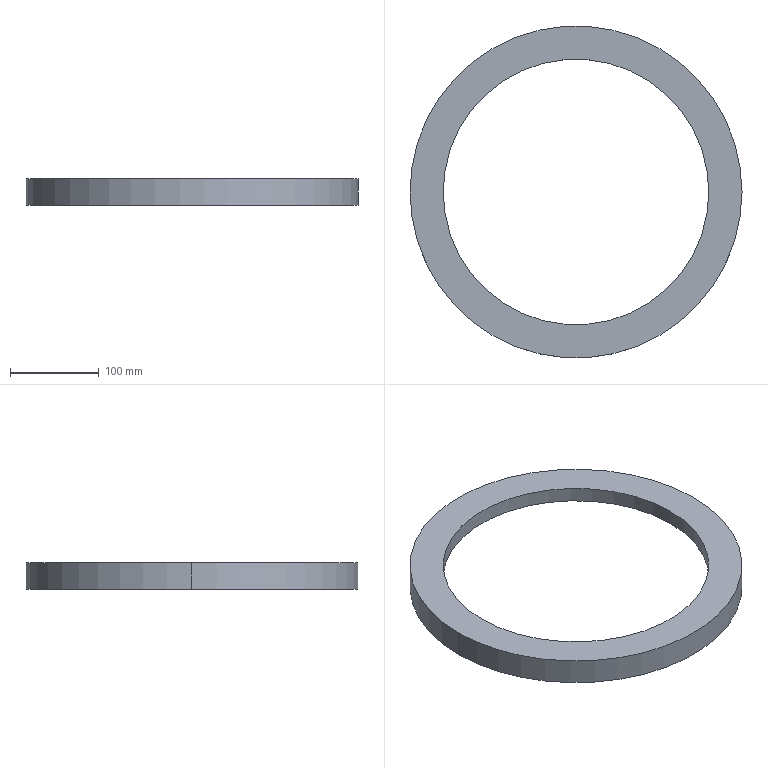Part | SolidWorks | features HoleWzd 1, Revolution 1 | 1 solid | 49 faces | box 375 x 375 x 30 mm | volume 842431 mm3 | cylinder 26 | cone 20 | plane 3 | commonest cylinder face diameters 6.8 x20 300 x2 352 x2 375 x2
STEP:
#1=CARTESIAN_POINT('',(3.4,162.5,-6.043));
#2=VERTEX_POINT('',#1);
#3=CARTESIAN_POINT('',(-3.4,162.5,-6.043));
#4=VERTEX_POINT('',#3);
#5=CARTESIAN_POINT('',(0.,162.5,-6.043));
#6=DIRECTION('',(0.,0.,-1.));
#7=DIRECTION('',(-1.,0.,0.));
#8=AXIS2_PLACEMENT_3D('',#5,#6,#7);
#9=CIRCLE('',#8,3.4);
#10=EDGE_CURVE('',#2,#4,#9,.T.);
#11=ORIENTED_EDGE('',*,*,#10,.F.);
#12=CARTESIAN_POINT('',(3.4,162.5,-17.));
#13=VERTEX_POINT('',#12);
#14=CARTESIAN_POINT('',(3.4,162.5,-17.));
#15=DIRECTION('',(0.,0.,-1.));
#16=VECTOR('',#15,1000.);
#17=LINE('',#14,#16);
#18=EDGE_CURVE('',#2,#13,#17,.T.);
#19=ORIENTED_EDGE('',*,*,#18,.T.);
#20=CARTESIAN_POINT('',(-3.4,162.5,-17.));
#21=VERTEX_POINT('',#20);
#22=CARTESIAN_POINT('',(0.,162.5,-17.));
#23=DIRECTION('',(0.,0.,-1.));
#24=DIRECTION('',(-1.,0.,0.));
#25=AXIS2_PLACEMENT_3D('',#22,#23,#24);
#26=CIRCLE('',#25,3.4);
#27=EDGE_CURVE('',#13,#21,#26,.T.);
#28=ORIENTED_EDGE('',*,*,#27,.T.);
#29=CARTESIAN_POINT('',(-3.4,162.5,-17.));
#30=DIRECTION('',(0.,0.,-1.));
#31=VECTOR('',#30,1000.);
#32=LINE('',#29,#31);
#33=EDGE_CURVE('',#4,#21,#32,.T.);
#34=ORIENTED_EDGE('',*,*,#33,.F.);
#35=EDGE_LOOP('',(#11,#19,#28,#34));
#36=FACE_OUTER_BOUND('',#35,.T.);
#37=CARTESIAN_POINT('',(0.,162.5,-17.));
#38=DIRECTION('',(0.,0.,-1.));
#39=DIRECTION('',(-1.,0.,0.));
#40=AXIS2_PLACEMENT_3D('',#37,#38,#39);
#41=CYLINDRICAL_SURFACE('',#40,3.4);
#42=ADVANCED_FACE('',(#36),#41,.F.);
#43=CARTESIAN_POINT('',(0.,162.5,-4.));
#44=VERTEX_POINT('',#43);
#45=CARTESIAN_POINT('',(-3.4,162.5,-6.043));
#46=DIRECTION('',(-0.8572,0.,-0.515));
#47=VECTOR('',#46,1000.);
#48=LINE('',#45,#47);
#49=EDGE_CURVE('',#44,#4,#48,.T.);
#50=ORIENTED_EDGE('',*,*,#49,.F.);
#51=CARTESIAN_POINT('',(3.4,162.5,-6.043));
#52=DIRECTION('',(0.8572,0.,-0.515));
#53=VECTOR('',#52,1000.);
#54=LINE('',#51,#53);
#55=EDGE_CURVE('',#44,#2,#54,.T.);
#56=ORIENTED_EDGE('',*,*,#55,.T.);
#57=ORIENTED_EDGE('',*,*,#10,.T.);
#58=EDGE_LOOP('',(#50,#56,#57));
#59=FACE_OUTER_BOUND('',#58,.T.);
#60=CARTESIAN_POINT('',(0.,162.5,-6.043));
#61=DIRECTION('',(0.,0.,-1.));
#62=DIRECTION('',(-1.,0.,0.));
#63=AXIS2_PLACEMENT_3D('',#60,#61,#62);
#64=CONICAL_SURFACE('',#63,3.4,1.03);
#65=ADVANCED_FACE('',(#59),#64,.F.);
#66=CARTESIAN_POINT('',(-92.115,131.465,-6.043));
#67=VERTEX_POINT('',#66);
#68=CARTESIAN_POINT('',(-98.915,131.465,-6.043));
#69=VERTEX_POINT('',#68);
#70=CARTESIAN_POINT('',(-95.515,131.465,-6.043));
#71=DIRECTION('',(0.,0.,-1.));
#72=DIRECTION('',(-1.,0.,0.));
#73=AXIS2_PLACEMENT_3D('',#70,#71,#72);
#74=CIRCLE('',#73,3.4);
#75=EDGE_CURVE('',#67,#69,#74,.T.);
#76=ORIENTED_EDGE('',*,*,#75,.F.);
#77=CARTESIAN_POINT('',(-92.115,131.465,-17.));
#78=VERTEX_POINT('',#77);
#79=CARTESIAN_POINT('',(-92.115,131.465,-17.));
#80=DIRECTION('',(0.,0.,-1.));
#81=VECTOR('',#80,1000.);
#82=LINE('',#79,#81);
#83=EDGE_CURVE('',#67,#78,#82,.T.);
#84=ORIENTED_EDGE('',*,*,#83,.T.);
#85=CARTESIAN_POINT('',(-98.915,131.465,-17.));
#86=VERTEX_POINT('',#85);
#87=CARTESIAN_POINT('',(-95.515,131.465,-17.));
#88=DIRECTION('',(0.,0.,-1.));
#89=DIRECTION('',(-1.,0.,0.));
#90=AXIS2_PLACEMENT_3D('',#87,#88,#89);
#91=CIRCLE('',#90,3.4);
#92=EDGE_CURVE('',#78,#86,#91,.T.);
#93=ORIENTED_EDGE('',*,*,#92,.T.);
#94=CARTESIAN_POINT('',(-98.915,131.465,-17.));
#95=DIRECTION('',(0.,0.,-1.));
#96=VECTOR('',#95,1000.);
#97=LINE('',#94,#96);
#98=EDGE_CURVE('',#69,#86,#97,.T.);
#99=ORIENTED_EDGE('',*,*,#98,.F.);
#100=EDGE_LOOP('',(#76,#84,#93,#99));
#101=FACE_OUTER_BOUND('',#100,.T.);
#102=CARTESIAN_POINT('',(-95.515,131.465,-17.));
#103=DIRECTION('',(0.,0.,-1.));
#104=DIRECTION('',(-1.,0.,0.));
#105=AXIS2_PLACEMENT_3D('',#102,#103,#104);
#106=CYLINDRICAL_SURFACE('',#105,3.4);
#107=ADVANCED_FACE('',(#101),#106,.F.);
#108=CARTESIAN_POINT('',(-95.515,131.465,-4.));
#109=VERTEX_POINT('',#108);
#110=CARTESIAN_POINT('',(-98.915,131.465,-6.043));
#111=DIRECTION('',(-0.8572,0.,-0.515));
#112=VECTOR('',#111,1000.);
#113=LINE('',#110,#112);
#114=EDGE_CURVE('',#109,#69,#113,.T.);
#115=ORIENTED_EDGE('',*,*,#114,.F.);
#116=CARTESIAN_POINT('',(-92.115,131.465,-6.043));
#117=DIRECTION('',(0.8572,0.,-0.515));
#118=VECTOR('',#117,1000.);
#119=LINE('',#116,#118);
#120=EDGE_CURVE('',#109,#67,#119,.T.);
#121=ORIENTED_EDGE('',*,*,#120,.T.);
#122=ORIENTED_EDGE('',*,*,#75,.T.);
#123=EDGE_LOOP('',(#115,#121,#122));
#124=FACE_OUTER_BOUND('',#123,.T.);
#125=CARTESIAN_POINT('',(-95.515,131.465,-6.043));
#126=DIRECTION('',(0.,0.,-1.));
#127=DIRECTION('',(-1.,0.,0.));
#128=AXIS2_PLACEMENT_3D('',#125,#126,#127);
#129=CONICAL_SURFACE('',#128,3.4,1.03);
#130=ADVANCED_FACE('',(#124),#129,.F.);
#131=CARTESIAN_POINT('',(-151.147,50.215,-6.043));
#132=VERTEX_POINT('',#131);
#133=CARTESIAN_POINT('',(-157.947,50.215,-6.043));
#134=VERTEX_POINT('',#133);
#135=CARTESIAN_POINT('',(-154.547,50.215,-6.043));
#136=DIRECTION('',(0.,0.,-1.));
#137=DIRECTION('',(-1.,0.,0.));
#138=AXIS2_PLACEMENT_3D('',#135,#136,#137);
#139=CIRCLE('',#138,3.4);
#140=EDGE_CURVE('',#132,#134,#139,.T.);
#141=ORIENTED_EDGE('',*,*,#140,.F.);
#142=CARTESIAN_POINT('',(-151.147,50.215,-17.));
#143=VERTEX_POINT('',#142);
#144=CARTESIAN_POINT('',(-151.147,50.215,-17.));
#145=DIRECTION('',(0.,0.,-1.));
#146=VECTOR('',#145,1000.);
#147=LINE('',#144,#146);
#148=EDGE_CURVE('',#132,#143,#147,.T.);
#149=ORIENTED_EDGE('',*,*,#148,.T.);
#150=CARTESIAN_POINT('',(-157.947,50.215,-17.));
#151=VERTEX_POINT('',#150);
#152=CARTESIAN_POINT('',(-154.547,50.215,-17.));
#153=DIRECTION('',(0.,0.,-1.));
#154=DIRECTION('',(-1.,0.,0.));
#155=AXIS2_PLACEMENT_3D('',#152,#153,#154);
#156=CIRCLE('',#155,3.4);
#157=EDGE_CURVE('',#143,#151,#156,.T.);
#158=ORIENTED_EDGE('',*,*,#157,.T.);
#159=CARTESIAN_POINT('',(-157.947,50.215,-17.));
#160=DIRECTION('',(0.,0.,-1.));
#161=VECTOR('',#160,1000.);
#162=LINE('',#159,#161);
#163=EDGE_CURVE('',#134,#151,#162,.T.);
#164=ORIENTED_EDGE('',*,*,#163,.F.);
#165=EDGE_LOOP('',(#141,#149,#158,#164));
#166=FACE_OUTER_BOUND('',#165,.T.);
#167=CARTESIAN_POINT('',(-154.547,50.215,-17.));
#168=DIRECTION('',(0.,0.,-1.));
#169=DIRECTION('',(-1.,0.,0.));
#170=AXIS2_PLACEMENT_3D('',#167,#168,#169);
#171=CYLINDRICAL_SURFACE('',#170,3.4);
#172=ADVANCED_FACE('',(#166),#171,.F.);
#173=CARTESIAN_POINT('',(-154.547,50.215,-4.));
#174=VERTEX_POINT('',#173);
#175=CARTESIAN_POINT('',(-157.947,50.215,-6.043));
#176=DIRECTION('',(-0.8572,0.,-0.515));
#177=VECTOR('',#176,1000.);
#178=LINE('',#175,#177);
#179=EDGE_CURVE('',#174,#134,#178,.T.);
#180=ORIENTED_EDGE('',*,*,#179,.F.);
#181=CARTESIAN_POINT('',(-151.147,50.215,-6.043));
#182=DIRECTION('',(0.8572,0.,-0.515));
#183=VECTOR('',#182,1000.);
#184=LINE('',#181,#183);
#185=EDGE_CURVE('',#174,#132,#184,.T.);
#186=ORIENTED_EDGE('',*,*,#185,.T.);
#187=ORIENTED_EDGE('',*,*,#140,.T.);
#188=EDGE_LOOP('',(#180,#186,#187));
#189=FACE_OUTER_BOUND('',#188,.T.);
#190=CARTESIAN_POINT('',(-154.547,50.215,-6.043));
#191=DIRECTION('',(0.,0.,-1.));
#192=DIRECTION('',(-1.,0.,0.));
#193=AXIS2_PLACEMENT_3D('',#190,#191,#192);
#194=CONICAL_SURFACE('',#193,3.4,1.03);
#195=ADVANCED_FACE('',(#189),#194,.F.);
#196=CARTESIAN_POINT('',(-151.147,-50.215,-6.043));
#197=VERTEX_POINT('',#196);
#198=CARTESIAN_POINT('',(-157.947,-50.215,-6.043));
#199=VERTEX_POINT('',#198);
#200=CARTESIAN_POINT('',(-154.547,-50.215,-6.043));
#201=DIRECTION('',(0.,0.,-1.));
#202=DIRECTION('',(-1.,0.,0.));
#203=AXIS2_PLACEMENT_3D('',#200,#201,#202);
#204=CIRCLE('',#203,3.4);
#205=EDGE_CURVE('',#197,#199,#204,.T.);
#206=ORIENTED_EDGE('',*,*,#205,.F.);
#207=CARTESIAN_POINT('',(-151.147,-50.215,-17.));
#208=VERTEX_POINT('',#207);
#209=CARTESIAN_POINT('',(-151.147,-50.215,-17.));
#210=DIRECTION('',(0.,0.,-1.));
#211=VECTOR('',#210,1000.);
#212=LINE('',#209,#211);
#213=EDGE_CURVE('',#197,#208,#212,.T.);
#214=ORIENTED_EDGE('',*,*,#213,.T.);
#215=CARTESIAN_POINT('',(-157.947,-50.215,-17.));
#216=VERTEX_POINT('',#215);
#217=CARTESIAN_POINT('',(-154.547,-50.215,-17.));
#218=DIRECTION('',(0.,0.,-1.));
#219=DIRECTION('',(-1.,0.,0.));
#220=AXIS2_PLACEMENT_3D('',#217,#218,#219);
#221=CIRCLE('',#220,3.4);
#222=EDGE_CURVE('',#208,#216,#221,.T.);
#223=ORIENTED_EDGE('',*,*,#222,.T.);
#224=CARTESIAN_POINT('',(-157.947,-50.215,-17.));
#225=DIRECTION('',(0.,0.,-1.));
#226=VECTOR('',#225,1000.);
#227=LINE('',#224,#226);
#228=EDGE_CURVE('',#199,#216,#227,.T.);
#229=ORIENTED_EDGE('',*,*,#228,.F.);
#230=EDGE_LOOP('',(#206,#214,#223,#229));
#231=FACE_OUTER_BOUND('',#230,.T.);
#232=CARTESIAN_POINT('',(-154.547,-50.215,-17.));
#233=DIRECTION('',(0.,0.,-1.));
#234=DIRECTION('',(-1.,0.,0.));
#235=AXIS2_PLACEMENT_3D('',#232,#233,#234);
#236=CYLINDRICAL_SURFACE('',#235,3.4);
#237=ADVANCED_FACE('',(#231),#236,.F.);
#238=CARTESIAN_POINT('',(-154.547,-50.215,-4.));
#239=VERTEX_POINT('',#238);
#240=CARTESIAN_POINT('',(-157.947,-50.215,-6.043));
#241=DIRECTION('',(-0.8572,0.,-0.515));
#242=VECTOR('',#241,1000.);
#243=LINE('',#240,#242);
#244=EDGE_CURVE('',#239,#199,#243,.T.);
#245=ORIENTED_EDGE('',*,*,#244,.F.);
#246=CARTESIAN_POINT('',(-151.147,-50.215,-6.043));
#247=DIRECTION('',(0.8572,0.,-0.515));
#248=VECTOR('',#247,1000.);
#249=LINE('',#246,#248);
#250=EDGE_CURVE('',#239,#197,#249,.T.);
#251=ORIENTED_EDGE('',*,*,#250,.T.);
#252=ORIENTED_EDGE('',*,*,#205,.T.);
#253=EDGE_LOOP('',(#245,#251,#252));
#254=FACE_OUTER_BOUND('',#253,.T.);
#255=CARTESIAN_POINT('',(-154.547,-50.215,-6.043));
#256=DIRECTION('',(0.,0.,-1.));
#257=DIRECTION('',(-1.,0.,0.));
#258=AXIS2_PLACEMENT_3D('',#255,#256,#257);
#259=CONICAL_SURFACE('',#258,3.4,1.03);
#260=ADVANCED_FACE('',(#254),#259,.F.);
#261=CARTESIAN_POINT('',(-92.115,-131.465,-6.043));
#262=VERTEX_POINT('',#261);
#263=CARTESIAN_POINT('',(-98.915,-131.465,-6.043));
#264=VERTEX_POINT('',#263);
#265=CARTESIAN_POINT('',(-95.515,-131.465,-6.043));
#266=DIRECTION('',(0.,0.,-1.));
#267=DIRECTION('',(-1.,0.,0.));
#268=AXIS2_PLACEMENT_3D('',#265,#266,#267);
#269=CIRCLE('',#268,3.4);
#270=EDGE_CURVE('',#262,#264,#269,.T.);
#271=ORIENTED_EDGE('',*,*,#270,.F.);
#272=CARTESIAN_POINT('',(-92.115,-131.465,-17.));
#273=VERTEX_POINT('',#272);
#274=CARTESIAN_POINT('',(-92.115,-131.465,-17.));
#275=DIRECTION('',(0.,0.,-1.));
#276=VECTOR('',#275,1000.);
#277=LINE('',#274,#276);
#278=EDGE_CURVE('',#262,#273,#277,.T.);
#279=ORIENTED_EDGE('',*,*,#278,.T.);
#280=CARTESIAN_POINT('',(-98.915,-131.465,-17.));
#281=VERTEX_POINT('',#280);
#282=CARTESIAN_POINT('',(-95.515,-131.465,-17.));
#283=DIRECTION('',(0.,0.,-1.));
#284=DIRECTION('',(-1.,0.,0.));
#285=AXIS2_PLACEMENT_3D('',#282,#283,#284);
#286=CIRCLE('',#285,3.4);
#287=EDGE_CURVE('',#273,#281,#286,.T.);
#288=ORIENTED_EDGE('',*,*,#287,.T.);
#289=CARTESIAN_POINT('',(-98.915,-131.465,-17.));
#290=DIRECTION('',(0.,0.,-1.));
#291=VECTOR('',#290,1000.);
#292=LINE('',#289,#291);
#293=EDGE_CURVE('',#264,#281,#292,.T.);
#294=ORIENTED_EDGE('',*,*,#293,.F.);
#295=EDGE_LOOP('',(#271,#279,#288,#294));
#296=FACE_OUTER_BOUND('',#295,.T.);
#297=CARTESIAN_POINT('',(-95.515,-131.465,-17.));
#298=DIRECTION('',(0.,0.,-1.));
#299=DIRECTION('',(-1.,0.,0.));
#300=AXIS2_PLACEMENT_3D('',#297,#298,#299);
#301=CYLINDRICAL_SURFACE('',#300,3.4);
#302=ADVANCED_FACE('',(#296),#301,.F.);
#303=CARTESIAN_POINT('',(-95.515,-131.465,-4.));
#304=VERTEX_POINT('',#303);
#305=CARTESIAN_POINT('',(-98.915,-131.465,-6.043));
#306=DIRECTION('',(-0.8572,0.,-0.515));
#307=VECTOR('',#306,1000.);
#308=LINE('',#305,#307);
#309=EDGE_CURVE('',#304,#264,#308,.T.);
#310=ORIENTED_EDGE('',*,*,#309,.F.);
#311=CARTESIAN_POINT('',(-92.115,-131.465,-6.043));
#312=DIRECTION('',(0.8572,0.,-0.515));
#313=VECTOR('',#312,1000.);
#314=LINE('',#311,#313);
#315=EDGE_CURVE('',#304,#262,#314,.T.);
#316=ORIENTED_EDGE('',*,*,#315,.T.);
#317=ORIENTED_EDGE('',*,*,#270,.T.);
#318=EDGE_LOOP('',(#310,#316,#317));
#319=FACE_OUTER_BOUND('',#318,.T.);
#320=CARTESIAN_POINT('',(-95.515,-131.465,-6.043));
#321=DIRECTION('',(0.,0.,-1.));
#322=DIRECTION('',(-1.,0.,0.));
#323=AXIS2_PLACEMENT_3D('',#320,#321,#322);
#324=CONICAL_SURFACE('',#323,3.4,1.03);
#325=ADVANCED_FACE('',(#319),#324,.F.);
#326=CARTESIAN_POINT('',(3.4,-162.5,-6.043));
#327=VERTEX_POINT('',#326);
#328=CARTESIAN_POINT('',(-3.4,-162.5,-6.043));
#329=VERTEX_POINT('',#328);
#330=CARTESIAN_POINT('',(0.,-162.5,-6.043));
#331=DIRECTION('',(0.,0.,-1.));
#332=DIRECTION('',(-1.,0.,0.));
#333=AXIS2_PLACEMENT_3D('',#330,#331,#332);
#334=CIRCLE('',#333,3.4);
#335=EDGE_CURVE('',#327,#329,#334,.T.);
#336=ORIENTED_EDGE('',*,*,#335,.F.);
#337=CARTESIAN_POINT('',(3.4,-162.5,-17.));
#338=VERTEX_POINT('',#337);
#339=CARTESIAN_POINT('',(3.4,-162.5,-17.));
#340=DIRECTION('',(0.,0.,-1.));
#341=VECTOR('',#340,1000.);
#342=LINE('',#339,#341);
#343=EDGE_CURVE('',#327,#338,#342,.T.);
#344=ORIENTED_EDGE('',*,*,#343,.T.);
#345=CARTESIAN_POINT('',(-3.4,-162.5,-17.));
#346=VERTEX_POINT('',#345);
#347=CARTESIAN_POINT('',(0.,-162.5,-17.));
#348=DIRECTION('',(0.,0.,-1.));
#349=DIRECTION('',(-1.,0.,0.));
#350=AXIS2_PLACEMENT_3D('',#347,#348,#349);
#351=CIRCLE('',#350,3.4);
#352=EDGE_CURVE('',#338,#346,#351,.T.);
#353=ORIENTED_EDGE('',*,*,#352,.T.);
#354=CARTESIAN_POINT('',(-3.4,-162.5,-17.));
#355=DIRECTION('',(0.,0.,-1.));
#356=VECTOR('',#355,1000.);
#357=LINE('',#354,#356);
#358=EDGE_CURVE('',#329,#346,#357,.T.);
#359=ORIENTED_EDGE('',*,*,#358,.F.);
#360=EDGE_LOOP('',(#336,#344,#353,#359));
#361=FACE_OUTER_BOUND('',#360,.T.);
#362=CARTESIAN_POINT('',(0.,-162.5,-17.));
#363=DIRECTION('',(0.,0.,-1.));
#364=DIRECTION('',(-1.,0.,0.));
#365=AXIS2_PLACEMENT_3D('',#362,#363,#364);
#366=CYLINDRICAL_SURFACE('',#365,3.4);
#367=ADVANCED_FACE('',(#361),#366,.F.);
#368=CARTESIAN_POINT('',(0.,-162.5,-4.));
#369=VERTEX_POINT('',#368);
#370=CARTESIAN_POINT('',(-3.4,-162.5,-6.043));
#371=DIRECTION('',(-0.8572,0.,-0.515));
#372=VECTOR('',#371,1000.);
#373=LINE('',#370,#372);
#374=EDGE_CURVE('',#369,#329,#373,.T.);
#375=ORIENTED_EDGE('',*,*,#374,.F.);
#376=CARTESIAN_POINT('',(3.4,-162.5,-6.043));
#377=DIRECTION('',(0.8572,0.,-0.515));
#378=VECTOR('',#377,1000.);
#379=LINE('',#376,#378);
#380=EDGE_CURVE('',#369,#327,#379,.T.);
#381=ORIENTED_EDGE('',*,*,#380,.T.);
#382=ORIENTED_EDGE('',*,*,#335,.T.);
#383=EDGE_LOOP('',(#375,#381,#382));
#384=FACE_OUTER_BOUND('',#383,.T.);
#385=CARTESIAN_POINT('',(0.,-162.5,-6.043));
#386=DIRECTION('',(0.,0.,-1.));
#387=DIRECTION('',(-1.,0.,0.));
#388=AXIS2_PLACEMENT_3D('',#385,#386,#387);
#389=CONICAL_SURFACE('',#388,3.4,1.03);
#390=ADVANCED_FACE('',(#384),#389,.F.);
#391=CARTESIAN_POINT('',(98.915,-131.465,-6.043));
#392=VERTEX_POINT('',#391);
#393=CARTESIAN_POINT('',(92.115,-131.465,-6.043));
#394=VERTEX_POINT('',#393);
#395=CARTESIAN_POINT('',(95.515,-131.465,-6.043));
#396=DIRECTION('',(0.,0.,-1.));
#397=DIRECTION('',(-1.,0.,0.));
#398=AXIS2_PLACEMENT_3D('',#395,#396,#397);
#399=CIRCLE('',#398,3.4);
#400=EDGE_CURVE('',#392,#394,#399,.T.);
#401=ORIENTED_EDGE('',*,*,#400,.F.);
#402=CARTESIAN_POINT('',(98.915,-131.465,-17.));
#403=VERTEX_POINT('',#402);
#404=CARTESIAN_POINT('',(98.915,-131.465,-17.));
#405=DIRECTION('',(0.,0.,-1.));
#406=VECTOR('',#405,1000.);
#407=LINE('',#404,#406);
#408=EDGE_CURVE('',#392,#403,#407,.T.);
#409=ORIENTED_EDGE('',*,*,#408,.T.);
#410=CARTESIAN_POINT('',(92.115,-131.465,-17.));
#411=VERTEX_POINT('',#410);
#412=CARTESIAN_POINT('',(95.515,-131.465,-17.));
#413=DIRECTION('',(0.,0.,-1.));
#414=DIRECTION('',(-1.,0.,0.));
#415=AXIS2_PLACEMENT_3D('',#412,#413,#414);
#416=CIRCLE('',#415,3.4);
#417=EDGE_CURVE('',#403,#411,#416,.T.);
#418=ORIENTED_EDGE('',*,*,#417,.T.);
#419=CARTESIAN_POINT('',(92.115,-131.465,-17.));
#420=DIRECTION('',(0.,0.,-1.));
#421=VECTOR('',#420,1000.);
#422=LINE('',#419,#421);
#423=EDGE_CURVE('',#394,#411,#422,.T.);
#424=ORIENTED_EDGE('',*,*,#423,.F.);
#425=EDGE_LOOP('',(#401,#409,#418,#424));
#426=FACE_OUTER_BOUND('',#425,.T.);
#427=CARTESIAN_POINT('',(95.515,-131.465,-17.));
#428=DIRECTION('',(0.,0.,-1.));
#429=DIRECTION('',(-1.,0.,0.));
#430=AXIS2_PLACEMENT_3D('',#427,#428,#429);
#431=CYLINDRICAL_SURFACE('',#430,3.4);
#432=ADVANCED_FACE('',(#426),#431,.F.);
#433=CARTESIAN_POINT('',(95.515,-131.465,-4.));
#434=VERTEX_POINT('',#433);
#435=CARTESIAN_POINT('',(92.115,-131.465,-6.043));
#436=DIRECTION('',(-0.8572,0.,-0.515));
#437=VECTOR('',#436,1000.);
#438=LINE('',#435,#437);
#439=EDGE_CURVE('',#434,#394,#438,.T.);
#440=ORIENTED_EDGE('',*,*,#439,.F.);
#441=CARTESIAN_POINT('',(98.915,-131.465,-6.043));
#442=DIRECTION('',(0.8572,0.,-0.515));
#443=VECTOR('',#442,1000.);
#444=LINE('',#441,#443);
#445=EDGE_CURVE('',#434,#392,#444,.T.);
#446=ORIENTED_EDGE('',*,*,#445,.T.);
#447=ORIENTED_EDGE('',*,*,#400,.T.);
#448=EDGE_LOOP('',(#440,#446,#447));
#449=FACE_OUTER_BOUND('',#448,.T.);
#450=CARTESIAN_POINT('',(95.515,-131.465,-6.043));
#451=DIRECTION('',(0.,0.,-1.));
#452=DIRECTION('',(-1.,0.,0.));
#453=AXIS2_PLACEMENT_3D('',#450,#451,#452);
#454=CONICAL_SURFACE('',#453,3.4,1.03);
#455=ADVANCED_FACE('',(#449),#454,.F.);
#456=CARTESIAN_POINT('',(157.947,-50.215,-6.043));
#457=VERTEX_POINT('',#456);
#458=CARTESIAN_POINT('',(151.147,-50.215,-6.043));
#459=VERTEX_POINT('',#458);
#460=CARTESIAN_POINT('',(154.547,-50.215,-6.043));
#461=DIRECTION('',(0.,0.,-1.));
#462=DIRECTION('',(-1.,0.,0.));
#463=AXIS2_PLACEMENT_3D('',#460,#461,#462);
#464=CIRCLE('',#463,3.4);
#465=EDGE_CURVE('',#457,#459,#464,.T.);
#466=ORIENTED_EDGE('',*,*,#465,.F.);
#467=CARTESIAN_POINT('',(157.947,-50.215,-17.));
#468=VERTEX_POINT('',#467);
#469=CARTESIAN_POINT('',(157.947,-50.215,-17.));
#470=DIRECTION('',(0.,0.,-1.));
#471=VECTOR('',#470,1000.);
#472=LINE('',#469,#471);
#473=EDGE_CURVE('',#457,#468,#472,.T.);
#474=ORIENTED_EDGE('',*,*,#473,.T.);
#475=CARTESIAN_POINT('',(151.147,-50.215,-17.));
#476=VERTEX_POINT('',#475);
#477=CARTESIAN_POINT('',(154.547,-50.215,-17.));
#478=DIRECTION('',(0.,0.,-1.));
#479=DIRECTION('',(-1.,0.,0.));
#480=AXIS2_PLACEMENT_3D('',#477,#478,#479);
#481=CIRCLE('',#480,3.4);
#482=EDGE_CURVE('',#468,#476,#481,.T.);
#483=ORIENTED_EDGE('',*,*,#482,.T.);
#484=CARTESIAN_POINT('',(151.147,-50.215,-17.));
#485=DIRECTION('',(0.,0.,-1.));
#486=VECTOR('',#485,1000.);
#487=LINE('',#484,#486);
#488=EDGE_CURVE('',#459,#476,#487,.T.);
#489=ORIENTED_EDGE('',*,*,#488,.F.);
#490=EDGE_LOOP('',(#466,#474,#483,#489));
#491=FACE_OUTER_BOUND('',#490,.T.);
#492=CARTESIAN_POINT('',(154.547,-50.215,-17.));
#493=DIRECTION('',(0.,0.,-1.));
#494=DIRECTION('',(-1.,0.,0.));
#495=AXIS2_PLACEMENT_3D('',#492,#493,#494);
#496=CYLINDRICAL_SURFACE('',#495,3.4);
#497=ADVANCED_FACE('',(#491),#496,.F.);
#498=CARTESIAN_POINT('',(154.547,-50.215,-4.));
#499=VERTEX_POINT('',#498);
#500=CARTESIAN_POINT('',(151.147,-50.215,-6.043));
#501=DIRECTION('',(-0.8572,0.,-0.515));
#502=VECTOR('',#501,1000.);
#503=LINE('',#500,#502);
#504=EDGE_CURVE('',#499,#459,#503,.T.);
#505=ORIENTED_EDGE('',*,*,#504,.F.);
#506=CARTESIAN_POINT('',(157.947,-50.215,-6.043));
#507=DIRECTION('',(0.8572,0.,-0.515));
#508=VECTOR('',#507,1000.);
#509=LINE('',#506,#508);
#510=EDGE_CURVE('',#499,#457,#509,.T.);
#511=ORIENTED_EDGE('',*,*,#510,.T.);
#512=ORIENTED_EDGE('',*,*,#465,.T.);
#513=EDGE_LOOP('',(#505,#511,#512));
#514=FACE_OUTER_BOUND('',#513,.T.);
#515=CARTESIAN_POINT('',(154.547,-50.215,-6.043));
#516=DIRECTION('',(0.,0.,-1.));
#517=DIRECTION('',(-1.,0.,0.));
#518=AXIS2_PLACEMENT_3D('',#515,#516,#517);
#519=CONICAL_SURFACE('',#518,3.4,1.03);
#520=ADVANCED_FACE('',(#514),#519,.F.);
#521=CARTESIAN_POINT('',(157.947,50.215,-6.043));
#522=VERTEX_POINT('',#521);
#523=CARTESIAN_POINT('',(151.147,50.215,-6.043));
#524=VERTEX_POINT('',#523);
#525=CARTESIAN_POINT('',(154.547,50.215,-6.043));
#526=DIRECTION('',(0.,0.,-1.));
#527=DIRECTION('',(-1.,0.,0.));
#528=AXIS2_PLACEMENT_3D('',#525,#526,#527);
#529=CIRCLE('',#528,3.4);
#530=EDGE_CURVE('',#522,#524,#529,.T.);
#531=ORIENTED_EDGE('',*,*,#530,.F.);
#532=CARTESIAN_POINT('',(157.947,50.215,-17.));
#533=VERTEX_POINT('',#532);
#534=CARTESIAN_POINT('',(157.947,50.215,-17.));
#535=DIRECTION('',(0.,0.,-1.));
#536=VECTOR('',#535,1000.);
#537=LINE('',#534,#536);
#538=EDGE_CURVE('',#522,#533,#537,.T.);
#539=ORIENTED_EDGE('',*,*,#538,.T.);
#540=CARTESIAN_POINT('',(151.147,50.215,-17.));
#541=VERTEX_POINT('',#540);
#542=CARTESIAN_POINT('',(154.547,50.215,-17.));
#543=DIRECTION('',(0.,0.,-1.));
#544=DIRECTION('',(-1.,0.,0.));
#545=AXIS2_PLACEMENT_3D('',#542,#543,#544);
#546=CIRCLE('',#545,3.4);
#547=EDGE_CURVE('',#533,#541,#546,.T.);
#548=ORIENTED_EDGE('',*,*,#547,.T.);
#549=CARTESIAN_POINT('',(151.147,50.215,-17.));
#550=DIRECTION('',(0.,0.,-1.));
#551=VECTOR('',#550,1000.);
#552=LINE('',#549,#551);
#553=EDGE_CURVE('',#524,#541,#552,.T.);
#554=ORIENTED_EDGE('',*,*,#553,.F.);
#555=EDGE_LOOP('',(#531,#539,#548,#554));
#556=FACE_OUTER_BOUND('',#555,.T.);
#557=CARTESIAN_POINT('',(154.547,50.215,-17.));
#558=DIRECTION('',(0.,0.,-1.));
#559=DIRECTION('',(-1.,0.,0.));
#560=AXIS2_PLACEMENT_3D('',#557,#558,#559);
#561=CYLINDRICAL_SURFACE('',#560,3.4);
#562=ADVANCED_FACE('',(#556),#561,.F.);
#563=CARTESIAN_POINT('',(154.547,50.215,-4.));
#564=VERTEX_POINT('',#563);
#565=CARTESIAN_POINT('',(151.147,50.215,-6.043));
#566=DIRECTION('',(-0.8572,0.,-0.515));
#567=VECTOR('',#566,1000.);
#568=LINE('',#565,#567);
#569=EDGE_CURVE('',#564,#524,#568,.T.);
#570=ORIENTED_EDGE('',*,*,#569,.F.);
#571=CARTESIAN_POINT('',(157.947,50.215,-6.043));
#572=DIRECTION('',(0.8572,0.,-0.515));
#573=VECTOR('',#572,1000.);
#574=LINE('',#571,#573);
#575=EDGE_CURVE('',#564,#522,#574,.T.);
#576=ORIENTED_EDGE('',*,*,#575,.T.);
#577=ORIENTED_EDGE('',*,*,#530,.T.);
#578=EDGE_LOOP('',(#570,#576,#577));
#579=FACE_OUTER_BOUND('',#578,.T.);
#580=CARTESIAN_POINT('',(154.547,50.215,-6.043));
#581=DIRECTION('',(0.,0.,-1.));
#582=DIRECTION('',(-1.,0.,0.));
#583=AXIS2_PLACEMENT_3D('',#580,#581,#582);
#584=CONICAL_SURFACE('',#583,3.4,1.03);
#585=ADVANCED_FACE('',(#579),#584,.F.);
#586=CARTESIAN_POINT('',(98.915,131.465,-6.043));
#587=VERTEX_POINT('',#586);
#588=CARTESIAN_POINT('',(92.115,131.465,-6.043));
#589=VERTEX_POINT('',#588);
#590=CARTESIAN_POINT('',(95.515,131.465,-6.043));
#591=DIRECTION('',(0.,0.,-1.));
#592=DIRECTION('',(-1.,0.,0.));
#593=AXIS2_PLACEMENT_3D('',#590,#591,#592);
#594=CIRCLE('',#593,3.4);
#595=EDGE_CURVE('',#587,#589,#594,.T.);
#596=ORIENTED_EDGE('',*,*,#595,.F.);
#597=CARTESIAN_POINT('',(98.915,131.465,-17.));
#598=VERTEX_POINT('',#597);
#599=CARTESIAN_POINT('',(98.915,131.465,-17.));
#600=DIRECTION('',(0.,0.,-1.));
#601=VECTOR('',#600,1000.);
#602=LINE('',#599,#601);
#603=EDGE_CURVE('',#587,#598,#602,.T.);
#604=ORIENTED_EDGE('',*,*,#603,.T.);
#605=CARTESIAN_POINT('',(92.115,131.465,-17.));
#606=VERTEX_POINT('',#605);
#607=CARTESIAN_POINT('',(95.515,131.465,-17.));
#608=DIRECTION('',(0.,0.,-1.));
#609=DIRECTION('',(-1.,0.,0.));
#610=AXIS2_PLACEMENT_3D('',#607,#608,#609);
#611=CIRCLE('',#610,3.4);
#612=EDGE_CURVE('',#598,#606,#611,.T.);
#613=ORIENTED_EDGE('',*,*,#612,.T.);
#614=CARTESIAN_POINT('',(92.115,131.465,-17.));
#615=DIRECTION('',(0.,0.,-1.));
#616=VECTOR('',#615,1000.);
#617=LINE('',#614,#616);
#618=EDGE_CURVE('',#589,#606,#617,.T.);
#619=ORIENTED_EDGE('',*,*,#618,.F.);
#620=EDGE_LOOP('',(#596,#604,#613,#619));
#621=FACE_OUTER_BOUND('',#620,.T.);
#622=CARTESIAN_POINT('',(95.515,131.465,-17.));
#623=DIRECTION('',(0.,0.,-1.));
#624=DIRECTION('',(-1.,0.,0.));
#625=AXIS2_PLACEMENT_3D('',#622,#623,#624);
#626=CYLINDRICAL_SURFACE('',#625,3.4);
#627=ADVANCED_FACE('',(#621),#626,.F.);
#628=CARTESIAN_POINT('',(95.515,131.465,-4.));
#629=VERTEX_POINT('',#628);
#630=CARTESIAN_POINT('',(92.115,131.465,-6.043));
#631=DIRECTION('',(-0.8572,0.,-0.515));
#632=VECTOR('',#631,1000.);
#633=LINE('',#630,#632);
#634=EDGE_CURVE('',#629,#589,#633,.T.);
#635=ORIENTED_EDGE('',*,*,#634,.F.);
#636=CARTESIAN_POINT('',(98.915,131.465,-6.043));
#637=DIRECTION('',(0.8572,0.,-0.515));
#638=VECTOR('',#637,1000.);
#639=LINE('',#636,#638);
#640=EDGE_CURVE('',#629,#587,#639,.T.);
#641=ORIENTED_EDGE('',*,*,#640,.T.);
#642=ORIENTED_EDGE('',*,*,#595,.T.);
#643=EDGE_LOOP('',(#635,#641,#642));
#644=FACE_OUTER_BOUND('',#643,.T.);
#645=CARTESIAN_POINT('',(95.515,131.465,-6.043));
#646=DIRECTION('',(0.,0.,-1.));
#647=DIRECTION('',(-1.,0.,0.));
#648=AXIS2_PLACEMENT_3D('',#645,#646,#647);
#649=CONICAL_SURFACE('',#648,3.4,1.03);
#650=ADVANCED_FACE('',(#644),#649,.F.);
#651=CARTESIAN_POINT('',(-150.,0.,-17.));
#652=VERTEX_POINT('',#651);
#653=CARTESIAN_POINT('',(150.,0.,-17.));
#654=VERTEX_POINT('',#653);
#655=CARTESIAN_POINT('',(0.,0.,-17.));
#656=DIRECTION('',(0.,0.,1.));
#657=DIRECTION('',(1.,0.,0.));
#658=AXIS2_PLACEMENT_3D('',#655,#656,#657);
#659=CIRCLE('',#658,150.);
#660=EDGE_CURVE('',#652,#654,#659,.T.);
#661=ORIENTED_EDGE('',*,*,#660,.F.);
#662=CARTESIAN_POINT('',(-150.,0.,0.));
#663=VERTEX_POINT('',#662);
#664=CARTESIAN_POINT('',(-150.,0.,0.));
#665=DIRECTION('',(0.,0.,1.));
#666=VECTOR('',#665,1000.);
#667=LINE('',#664,#666);
#668=EDGE_CURVE('',#652,#663,#667,.T.);
#669=ORIENTED_EDGE('',*,*,#668,.T.);
#670=CARTESIAN_POINT('',(150.,0.,0.));
#671=VERTEX_POINT('',#670);
#672=CARTESIAN_POINT('',(0.,0.,0.));
#673=DIRECTION('',(0.,0.,1.));
#674=DIRECTION('',(1.,0.,0.));
#675=AXIS2_PLACEMENT_3D('',#672,#673,#674);
#676=CIRCLE('',#675,150.);
#677=EDGE_CURVE('',#663,#671,#676,.T.);
#678=ORIENTED_EDGE('',*,*,#677,.T.);
#679=CARTESIAN_POINT('',(150.,0.,0.));
#680=DIRECTION('',(0.,0.,1.));
#681=VECTOR('',#680,1000.);
#682=LINE('',#679,#681);
#683=EDGE_CURVE('',#654,#671,#682,.T.);
#684=ORIENTED_EDGE('',*,*,#683,.F.);
#685=EDGE_LOOP('',(#661,#669,#678,#684));
#686=FACE_OUTER_BOUND('',#685,.T.);
#687=CARTESIAN_POINT('',(0.,0.,0.));
#688=DIRECTION('',(0.,0.,1.));
#689=DIRECTION('',(1.,0.,0.));
#690=AXIS2_PLACEMENT_3D('',#687,#688,#689);
#691=CYLINDRICAL_SURFACE('',#690,150.);
#692=ADVANCED_FACE('',(#686),#691,.F.);
#693=CARTESIAN_POINT('',(-176.,0.,-30.));
#694=VERTEX_POINT('',#693);
#695=CARTESIAN_POINT('',(176.,0.,-30.));
#696=VERTEX_POINT('',#695);
#697=CARTESIAN_POINT('',(0.,0.,-30.));
#698=DIRECTION('',(0.,0.,1.));
#699=DIRECTION('',(1.,0.,0.));
#700=AXIS2_PLACEMENT_3D('',#697,#698,#699);
#701=CIRCLE('',#700,176.);
#702=EDGE_CURVE('',#694,#696,#701,.T.);
#703=ORIENTED_EDGE('',*,*,#702,.F.);
#704=CARTESIAN_POINT('',(-176.,0.,-17.));
#705=VERTEX_POINT('',#704);
#706=CARTESIAN_POINT('',(-176.,0.,0.));
#707=DIRECTION('',(0.,0.,1.));
#708=VECTOR('',#707,1000.);
#709=LINE('',#706,#708);
#710=EDGE_CURVE('',#694,#705,#709,.T.);
#711=ORIENTED_EDGE('',*,*,#710,.T.);
#712=CARTESIAN_POINT('',(176.,0.,-17.));
#713=VERTEX_POINT('',#712);
#714=CARTESIAN_POINT('',(0.,0.,-17.));
#715=DIRECTION('',(0.,0.,1.));
#716=DIRECTION('',(1.,0.,0.));
#717=AXIS2_PLACEMENT_3D('',#714,#715,#716);
#718=CIRCLE('',#717,176.);
#719=EDGE_CURVE('',#705,#713,#718,.T.);
#720=ORIENTED_EDGE('',*,*,#719,.T.);
#721=CARTESIAN_POINT('',(176.,0.,0.));
#722=DIRECTION('',(0.,0.,1.));
#723=VECTOR('',#722,1000.);
#724=LINE('',#721,#723);
#725=EDGE_CURVE('',#696,#713,#724,.T.);
#726=ORIENTED_EDGE('',*,*,#725,.F.);
#727=EDGE_LOOP('',(#703,#711,#720,#726));
#728=FACE_OUTER_BOUND('',#727,.T.);
#729=CARTESIAN_POINT('',(0.,0.,0.));
#730=DIRECTION('',(0.,0.,1.));
#731=DIRECTION('',(1.,0.,0.));
#732=AXIS2_PLACEMENT_3D('',#729,#730,#731);
#733=CYLINDRICAL_SURFACE('',#732,176.);
#734=ADVANCED_FACE('',(#728),#733,.F.);
#735=CARTESIAN_POINT('',(187.5,0.,-30.));
#736=VERTEX_POINT('',#735);
#737=CARTESIAN_POINT('',(-187.5,0.,-30.));
#738=VERTEX_POINT('',#737);
#739=CARTESIAN_POINT('',(0.,0.,-30.));
#740=DIRECTION('',(0.,0.,1.));
#741=DIRECTION('',(1.,0.,0.));
#742=AXIS2_PLACEMENT_3D('',#739,#740,#741);
#743=CIRCLE('',#742,187.5);
#744=EDGE_CURVE('',#736,#738,#743,.T.);
#745=ORIENTED_EDGE('',*,*,#744,.T.);
#746=CARTESIAN_POINT('',(-187.5,0.,0.));
#747=VERTEX_POINT('',#746);
#748=CARTESIAN_POINT('',(-187.5,0.,0.));
#749=DIRECTION('',(0.,0.,1.));
#750=VECTOR('',#749,1000.);
#751=LINE('',#748,#750);
#752=EDGE_CURVE('',#738,#747,#751,.T.);
#753=ORIENTED_EDGE('',*,*,#752,.T.);
#754=CARTESIAN_POINT('',(187.5,0.,0.));
#755=VERTEX_POINT('',#754);
#756=CARTESIAN_POINT('',(0.,0.,0.));
#757=DIRECTION('',(0.,0.,1.));
#758=DIRECTION('',(1.,0.,0.));
#759=AXIS2_PLACEMENT_3D('',#756,#757,#758);
#760=CIRCLE('',#759,187.5);
#761=EDGE_CURVE('',#755,#747,#760,.T.);
#762=ORIENTED_EDGE('',*,*,#761,.F.);
#763=CARTESIAN_POINT('',(187.5,0.,0.));
#764=DIRECTION('',(0.,0.,1.));
#765=VECTOR('',#764,1000.);
#766=LINE('',#763,#765);
#767=EDGE_CURVE('',#736,#755,#766,.T.);
#768=ORIENTED_EDGE('',*,*,#767,.F.);
#769=EDGE_LOOP('',(#745,#753,#762,#768));
#770=FACE_OUTER_BOUND('',#769,.T.);
#771=CARTESIAN_POINT('',(0.,0.,0.));
#772=DIRECTION('',(0.,0.,1.));
#773=DIRECTION('',(1.,0.,0.));
#774=AXIS2_PLACEMENT_3D('',#771,#772,#773);
#775=CYLINDRICAL_SURFACE('',#774,187.5);
#776=ADVANCED_FACE('',(#770),#775,.T.);
#777=ORIENTED_EDGE('',*,*,#752,.F.);
#778=CARTESIAN_POINT('',(0.,0.,-30.));
#779=DIRECTION('',(0.,0.,1.));
#780=DIRECTION('',(1.,0.,0.));
#781=AXIS2_PLACEMENT_3D('',#778,#779,#780);
#782=CIRCLE('',#781,187.5);
#783=EDGE_CURVE('',#738,#736,#782,.T.);
#784=ORIENTED_EDGE('',*,*,#783,.T.);
#785=ORIENTED_EDGE('',*,*,#767,.T.);
#786=CARTESIAN_POINT('',(0.,0.,0.));
#787=DIRECTION('',(0.,0.,1.));
#788=DIRECTION('',(1.,0.,0.));
#789=AXIS2_PLACEMENT_3D('',#786,#787,#788);
#790=CIRCLE('',#789,187.5);
#791=EDGE_CURVE('',#747,#755,#790,.T.);
#792=ORIENTED_EDGE('',*,*,#791,.F.);
#793=EDGE_LOOP('',(#777,#784,#785,#792));
#794=FACE_OUTER_BOUND('',#793,.T.);
#795=CARTESIAN_POINT('',(0.,0.,0.));
#796=DIRECTION('',(0.,0.,1.));
#797=DIRECTION('',(1.,0.,0.));
#798=AXIS2_PLACEMENT_3D('',#795,#796,#797);
#799=CYLINDRICAL_SURFACE('',#798,187.5);
#800=ADVANCED_FACE('',(#794),#799,.T.);
#801=ORIENTED_EDGE('',*,*,#744,.F.);
#802=ORIENTED_EDGE('',*,*,#783,.F.);
#803=EDGE_LOOP('',(#801,#802));
#804=FACE_OUTER_BOUND('',#803,.T.);
#805=CARTESIAN_POINT('',(0.,0.,-30.));
#806=DIRECTION('',(0.,0.,1.));
#807=DIRECTION('',(1.,0.,0.));
#808=AXIS2_PLACEMENT_3D('',#805,#806,#807);
#809=CIRCLE('',#808,176.);
#810=EDGE_CURVE('',#696,#694,#809,.T.);
#811=ORIENTED_EDGE('',*,*,#810,.T.);
#812=ORIENTED_EDGE('',*,*,#702,.T.);
#813=EDGE_LOOP('',(#811,#812));
#814=FACE_BOUND('',#813,.T.);
#815=CARTESIAN_POINT('',(0.,187.5,-30.));
#816=DIRECTION('',(0.,0.,1.));
#817=DIRECTION('',(1.,0.,0.));
#818=AXIS2_PLACEMENT_3D('',#815,#816,#817);
#819=PLANE('',#818);
#820=ADVANCED_FACE('',(#804,#814),#819,.F.);
#821=ORIENTED_EDGE('',*,*,#710,.F.);
#822=ORIENTED_EDGE('',*,*,#810,.F.);
#823=ORIENTED_EDGE('',*,*,#725,.T.);
#824=CARTESIAN_POINT('',(0.,0.,-17.));
#825=DIRECTION('',(0.,0.,1.));
#826=DIRECTION('',(1.,0.,0.));
#827=AXIS2_PLACEMENT_3D('',#824,#825,#826);
#828=CIRCLE('',#827,176.);
#829=EDGE_CURVE('',#713,#705,#828,.T.);
#830=ORIENTED_EDGE('',*,*,#829,.T.);
#831=EDGE_LOOP('',(#821,#822,#823,#830));
#832=FACE_OUTER_BOUND('',#831,.T.);
#833=CARTESIAN_POINT('',(0.,0.,0.));
#834=DIRECTION('',(0.,0.,1.));
#835=DIRECTION('',(1.,0.,0.));
#836=AXIS2_PLACEMENT_3D('',#833,#834,#835);
#837=CYLINDRICAL_SURFACE('',#836,176.);
#838=ADVANCED_FACE('',(#832),#837,.F.);
#839=CARTESIAN_POINT('',(0.,162.5,-17.));
#840=DIRECTION('',(0.,0.,-1.));
#841=DIRECTION('',(-1.,0.,0.));
#842=AXIS2_PLACEMENT_3D('',#839,#840,#841);
#843=CIRCLE('',#842,3.4);
#844=EDGE_CURVE('',#21,#13,#843,.T.);
#845=ORIENTED_EDGE('',*,*,#844,.F.);
#846=ORIENTED_EDGE('',*,*,#27,.F.);
#847=EDGE_LOOP('',(#845,#846));
#848=FACE_BOUND('',#847,.T.);
#849=CARTESIAN_POINT('',(-95.515,131.465,-17.));
#850=DIRECTION('',(0.,0.,-1.));
#851=DIRECTION('',(-1.,0.,0.));
#852=AXIS2_PLACEMENT_3D('',#849,#850,#851);
#853=CIRCLE('',#852,3.4);
#854=EDGE_CURVE('',#86,#78,#853,.T.);
#855=ORIENTED_EDGE('',*,*,#854,.F.);
#856=ORIENTED_EDGE('',*,*,#92,.F.);
#857=EDGE_LOOP('',(#855,#856));
#858=FACE_BOUND('',#857,.T.);
#859=CARTESIAN_POINT('',(-154.547,50.215,-17.));
#860=DIRECTION('',(0.,0.,-1.));
#861=DIRECTION('',(-1.,0.,0.));
#862=AXIS2_PLACEMENT_3D('',#859,#860,#861);
#863=CIRCLE('',#862,3.4);
#864=EDGE_CURVE('',#151,#143,#863,.T.);
#865=ORIENTED_EDGE('',*,*,#864,.F.);
#866=ORIENTED_EDGE('',*,*,#157,.F.);
#867=EDGE_LOOP('',(#865,#866));
#868=FACE_BOUND('',#867,.T.);
#869=CARTESIAN_POINT('',(-154.547,-50.215,-17.));
#870=DIRECTION('',(0.,0.,-1.));
#871=DIRECTION('',(-1.,0.,0.));
#872=AXIS2_PLACEMENT_3D('',#869,#870,#871);
#873=CIRCLE('',#872,3.4);
#874=EDGE_CURVE('',#216,#208,#873,.T.);
#875=ORIENTED_EDGE('',*,*,#874,.F.);
#876=ORIENTED_EDGE('',*,*,#222,.F.);
#877=EDGE_LOOP('',(#875,#876));
#878=FACE_BOUND('',#877,.T.);
#879=CARTESIAN_POINT('',(-95.515,-131.465,-17.));
#880=DIRECTION('',(0.,0.,-1.));
#881=DIRECTION('',(-1.,0.,0.));
#882=AXIS2_PLACEMENT_3D('',#879,#880,#881);
#883=CIRCLE('',#882,3.4);
#884=EDGE_CURVE('',#281,#273,#883,.T.);
#885=ORIENTED_EDGE('',*,*,#884,.F.);
#886=ORIENTED_EDGE('',*,*,#287,.F.);
#887=EDGE_LOOP('',(#885,#886));
#888=FACE_BOUND('',#887,.T.);
#889=CARTESIAN_POINT('',(0.,-162.5,-17.));
#890=DIRECTION('',(0.,0.,-1.));
#891=DIRECTION('',(-1.,0.,0.));
#892=AXIS2_PLACEMENT_3D('',#889,#890,#891);
#893=CIRCLE('',#892,3.4);
#894=EDGE_CURVE('',#346,#338,#893,.T.);
#895=ORIENTED_EDGE('',*,*,#894,.F.);
#896=ORIENTED_EDGE('',*,*,#352,.F.);
#897=EDGE_LOOP('',(#895,#896));
#898=FACE_BOUND('',#897,.T.);
#899=CARTESIAN_POINT('',(95.515,-131.465,-17.));
#900=DIRECTION('',(0.,0.,-1.));
#901=DIRECTION('',(-1.,0.,0.));
#902=AXIS2_PLACEMENT_3D('',#899,#900,#901);
#903=CIRCLE('',#902,3.4);
#904=EDGE_CURVE('',#411,#403,#903,.T.);
#905=ORIENTED_EDGE('',*,*,#904,.F.);
#906=ORIENTED_EDGE('',*,*,#417,.F.);
#907=EDGE_LOOP('',(#905,#906));
#908=FACE_BOUND('',#907,.T.);
#909=CARTESIAN_POINT('',(154.547,-50.215,-17.));
#910=DIRECTION('',(0.,0.,-1.));
#911=DIRECTION('',(-1.,0.,0.));
#912=AXIS2_PLACEMENT_3D('',#909,#910,#911);
#913=CIRCLE('',#912,3.4);
#914=EDGE_CURVE('',#476,#468,#913,.T.);
#915=ORIENTED_EDGE('',*,*,#914,.F.);
#916=ORIENTED_EDGE('',*,*,#482,.F.);
#917=EDGE_LOOP('',(#915,#916));
#918=FACE_BOUND('',#917,.T.);
#919=CARTESIAN_POINT('',(154.547,50.215,-17.));
#920=DIRECTION('',(0.,0.,-1.));
#921=DIRECTION('',(-1.,0.,0.));
#922=AXIS2_PLACEMENT_3D('',#919,#920,#921);
#923=CIRCLE('',#922,3.4);
#924=EDGE_CURVE('',#541,#533,#923,.T.);
#925=ORIENTED_EDGE('',*,*,#924,.F.);
#926=ORIENTED_EDGE('',*,*,#547,.F.);
#927=EDGE_LOOP('',(#925,#926));
#928=FACE_BOUND('',#927,.T.);
#929=CARTESIAN_POINT('',(95.515,131.465,-17.));
#930=DIRECTION('',(0.,0.,-1.));
#931=DIRECTION('',(-1.,0.,0.));
#932=AXIS2_PLACEMENT_3D('',#929,#930,#931);
#933=CIRCLE('',#932,3.4);
#934=EDGE_CURVE('',#606,#598,#933,.T.);
#935=ORIENTED_EDGE('',*,*,#934,.F.);
#936=ORIENTED_EDGE('',*,*,#612,.F.);
#937=EDGE_LOOP('',(#935,#936));
#938=FACE_BOUND('',#937,.T.);
#939=ORIENTED_EDGE('',*,*,#829,.F.);
#940=ORIENTED_EDGE('',*,*,#719,.F.);
#941=EDGE_LOOP('',(#939,#940));
#942=FACE_OUTER_BOUND('',#941,.T.);
#943=CARTESIAN_POINT('',(0.,0.,-17.));
#944=DIRECTION('',(0.,0.,1.));
#945=DIRECTION('',(1.,0.,0.));
#946=AXIS2_PLACEMENT_3D('',#943,#944,#945);
#947=CIRCLE('',#946,150.);
#948=EDGE_CURVE('',#654,#652,#947,.T.);
#949=ORIENTED_EDGE('',*,*,#948,.T.);
#950=ORIENTED_EDGE('',*,*,#660,.T.);
#951=EDGE_LOOP('',(#949,#950));
#952=FACE_BOUND('',#951,.T.);
#953=CARTESIAN_POINT('',(0.,176.,-17.));
#954=DIRECTION('',(0.,0.,1.));
#955=DIRECTION('',(1.,0.,0.));
#956=AXIS2_PLACEMENT_3D('',#953,#954,#955);
#957=PLANE('',#956);
#958=ADVANCED_FACE('',(#848,#858,#868,#878,#888,#898,#908,#918,#928,#938,#942,#952),#957,.F.);
#959=ORIENTED_EDGE('',*,*,#668,.F.);
#960=ORIENTED_EDGE('',*,*,#948,.F.);
#961=ORIENTED_EDGE('',*,*,#683,.T.);
#962=CARTESIAN_POINT('',(0.,0.,0.));
#963=DIRECTION('',(0.,0.,1.));
#964=DIRECTION('',(1.,0.,0.));
#965=AXIS2_PLACEMENT_3D('',#962,#963,#964);
#966=CIRCLE('',#965,150.);
#967=EDGE_CURVE('',#671,#663,#966,.T.);
#968=ORIENTED_EDGE('',*,*,#967,.T.);
#969=EDGE_LOOP('',(#959,#960,#961,#968));
#970=FACE_OUTER_BOUND('',#969,.T.);
#971=CARTESIAN_POINT('',(0.,0.,0.));
#972=DIRECTION('',(0.,0.,1.));
#973=DIRECTION('',(1.,0.,0.));
#974=AXIS2_PLACEMENT_3D('',#971,#972,#973);
#975=CYLINDRICAL_SURFACE('',#974,150.);
#976=ADVANCED_FACE('',(#970),#975,.F.);
#977=ORIENTED_EDGE('',*,*,#967,.F.);
#978=ORIENTED_EDGE('',*,*,#677,.F.);
#979=EDGE_LOOP('',(#977,#978));
#980=FACE_BOUND('',#979,.T.);
#981=ORIENTED_EDGE('',*,*,#761,.T.);
#982=ORIENTED_EDGE('',*,*,#791,.T.);
#983=EDGE_LOOP('',(#981,#982));
#984=FACE_OUTER_BOUND('',#983,.T.);
#985=CARTESIAN_POINT('',(0.,150.,0.));
#986=DIRECTION('',(0.,0.,-1.));
#987=DIRECTION('',(-1.,0.,0.));
#988=AXIS2_PLACEMENT_3D('',#985,#986,#987);
#989=PLANE('',#988);
#990=ADVANCED_FACE('',(#980,#984),#989,.F.);
#991=ORIENTED_EDGE('',*,*,#640,.F.);
#992=ORIENTED_EDGE('',*,*,#634,.T.);
#993=CARTESIAN_POINT('',(95.515,131.465,-6.043));
#994=DIRECTION('',(0.,0.,-1.));
#995=DIRECTION('',(-1.,0.,0.));
#996=AXIS2_PLACEMENT_3D('',#993,#994,#995);
#997=CIRCLE('',#996,3.4);
#998=EDGE_CURVE('',#589,#587,#997,.T.);
#999=ORIENTED_EDGE('',*,*,#998,.T.);
#1000=EDGE_LOOP('',(#991,#992,#999));
#1001=FACE_OUTER_BOUND('',#1000,.T.);
#1002=CARTESIAN_POINT('',(95.515,131.465,-6.043));
#1003=DIRECTION('',(0.,0.,-1.));
#1004=DIRECTION('',(-1.,0.,0.));
#1005=AXIS2_PLACEMENT_3D('',#1002,#1003,#1004);
#1006=CONICAL_SURFACE('',#1005,3.4,1.03);
#1007=ADVANCED_FACE('',(#1001),#1006,.F.);
#1008=ORIENTED_EDGE('',*,*,#603,.F.);
#1009=ORIENTED_EDGE('',*,*,#998,.F.);
#1010=ORIENTED_EDGE('',*,*,#618,.T.);
#1011=ORIENTED_EDGE('',*,*,#934,.T.);
#1012=EDGE_LOOP('',(#1008,#1009,#1010,#1011));
#1013=FACE_OUTER_BOUND('',#1012,.T.);
#1014=CARTESIAN_POINT('',(95.515,131.465,-17.));
#1015=DIRECTION('',(0.,0.,-1.));
#1016=DIRECTION('',(-1.,0.,0.));
#1017=AXIS2_PLACEMENT_3D('',#1014,#1015,#1016);
#1018=CYLINDRICAL_SURFACE('',#1017,3.4);
#1019=ADVANCED_FACE('',(#1013),#1018,.F.);
#1020=ORIENTED_EDGE('',*,*,#575,.F.);
#1021=ORIENTED_EDGE('',*,*,#569,.T.);
#1022=CARTESIAN_POINT('',(154.547,50.215,-6.043));
#1023=DIRECTION('',(0.,0.,-1.));
#1024=DIRECTION('',(-1.,0.,0.));
#1025=AXIS2_PLACEMENT_3D('',#1022,#1023,#1024);
#1026=CIRCLE('',#1025,3.4);
#1027=EDGE_CURVE('',#524,#522,#1026,.T.);
#1028=ORIENTED_EDGE('',*,*,#1027,.T.);
#1029=EDGE_LOOP('',(#1020,#1021,#1028));
#1030=FACE_OUTER_BOUND('',#1029,.T.);
#1031=CARTESIAN_POINT('',(154.547,50.215,-6.043));
#1032=DIRECTION('',(0.,0.,-1.));
#1033=DIRECTION('',(-1.,0.,0.));
#1034=AXIS2_PLACEMENT_3D('',#1031,#1032,#1033);
#1035=CONICAL_SURFACE('',#1034,3.4,1.03);
#1036=ADVANCED_FACE('',(#1030),#1035,.F.);
#1037=ORIENTED_EDGE('',*,*,#538,.F.);
#1038=ORIENTED_EDGE('',*,*,#1027,.F.);
#1039=ORIENTED_EDGE('',*,*,#553,.T.);
#1040=ORIENTED_EDGE('',*,*,#924,.T.);
#1041=EDGE_LOOP('',(#1037,#1038,#1039,#1040));
#1042=FACE_OUTER_BOUND('',#1041,.T.);
#1043=CARTESIAN_POINT('',(154.547,50.215,-17.));
#1044=DIRECTION('',(0.,0.,-1.));
#1045=DIRECTION('',(-1.,0.,0.));
#1046=AXIS2_PLACEMENT_3D('',#1043,#1044,#1045);
#1047=CYLINDRICAL_SURFACE('',#1046,3.4);
#1048=ADVANCED_FACE('',(#1042),#1047,.F.);
#1049=ORIENTED_EDGE('',*,*,#510,.F.);
#1050=ORIENTED_EDGE('',*,*,#504,.T.);
#1051=CARTESIAN_POINT('',(154.547,-50.215,-6.043));
#1052=DIRECTION('',(0.,0.,-1.));
#1053=DIRECTION('',(-1.,0.,0.));
#1054=AXIS2_PLACEMENT_3D('',#1051,#1052,#1053);
#1055=CIRCLE('',#1054,3.4);
#1056=EDGE_CURVE('',#459,#457,#1055,.T.);
#1057=ORIENTED_EDGE('',*,*,#1056,.T.);
#1058=EDGE_LOOP('',(#1049,#1050,#1057));
#1059=FACE_OUTER_BOUND('',#1058,.T.);
#1060=CARTESIAN_POINT('',(154.547,-50.215,-6.043));
#1061=DIRECTION('',(0.,0.,-1.));
#1062=DIRECTION('',(-1.,0.,0.));
#1063=AXIS2_PLACEMENT_3D('',#1060,#1061,#1062);
#1064=CONICAL_SURFACE('',#1063,3.4,1.03);
#1065=ADVANCED_FACE('',(#1059),#1064,.F.);
#1066=ORIENTED_EDGE('',*,*,#473,.F.);
#1067=ORIENTED_EDGE('',*,*,#1056,.F.);
#1068=ORIENTED_EDGE('',*,*,#488,.T.);
#1069=ORIENTED_EDGE('',*,*,#914,.T.);
#1070=EDGE_LOOP('',(#1066,#1067,#1068,#1069));
#1071=FACE_OUTER_BOUND('',#1070,.T.);
#1072=CARTESIAN_POINT('',(154.547,-50.215,-17.));
#1073=DIRECTION('',(0.,0.,-1.));
#1074=DIRECTION('',(-1.,0.,0.));
#1075=AXIS2_PLACEMENT_3D('',#1072,#1073,#1074);
#1076=CYLINDRICAL_SURFACE('',#1075,3.4);
#1077=ADVANCED_FACE('',(#1071),#1076,.F.);
#1078=ORIENTED_EDGE('',*,*,#445,.F.);
#1079=ORIENTED_EDGE('',*,*,#439,.T.);
#1080=CARTESIAN_POINT('',(95.515,-131.465,-6.043));
#1081=DIRECTION('',(0.,0.,-1.));
#1082=DIRECTION('',(-1.,0.,0.));
#1083=AXIS2_PLACEMENT_3D('',#1080,#1081,#1082);
#1084=CIRCLE('',#1083,3.4);
#1085=EDGE_CURVE('',#394,#392,#1084,.T.);
#1086=ORIENTED_EDGE('',*,*,#1085,.T.);
#1087=EDGE_LOOP('',(#1078,#1079,#1086));
#1088=FACE_OUTER_BOUND('',#1087,.T.);
#1089=CARTESIAN_POINT('',(95.515,-131.465,-6.043));
#1090=DIRECTION('',(0.,0.,-1.));
#1091=DIRECTION('',(-1.,0.,0.));
#1092=AXIS2_PLACEMENT_3D('',#1089,#1090,#1091);
#1093=CONICAL_SURFACE('',#1092,3.4,1.03);
#1094=ADVANCED_FACE('',(#1088),#1093,.F.);
#1095=ORIENTED_EDGE('',*,*,#408,.F.);
#1096=ORIENTED_EDGE('',*,*,#1085,.F.);
#1097=ORIENTED_EDGE('',*,*,#423,.T.);
#1098=ORIENTED_EDGE('',*,*,#904,.T.);
#1099=EDGE_LOOP('',(#1095,#1096,#1097,#1098));
#1100=FACE_OUTER_BOUND('',#1099,.T.);
#1101=CARTESIAN_POINT('',(95.515,-131.465,-17.));
#1102=DIRECTION('',(0.,0.,-1.));
#1103=DIRECTION('',(-1.,0.,0.));
#1104=AXIS2_PLACEMENT_3D('',#1101,#1102,#1103);
#1105=CYLINDRICAL_SURFACE('',#1104,3.4);
#1106=ADVANCED_FACE('',(#1100),#1105,.F.);
#1107=ORIENTED_EDGE('',*,*,#380,.F.);
#1108=ORIENTED_EDGE('',*,*,#374,.T.);
#1109=CARTESIAN_POINT('',(0.,-162.5,-6.043));
#1110=DIRECTION('',(0.,0.,-1.));
#1111=DIRECTION('',(-1.,0.,0.));
#1112=AXIS2_PLACEMENT_3D('',#1109,#1110,#1111);
#1113=CIRCLE('',#1112,3.4);
#1114=EDGE_CURVE('',#329,#327,#1113,.T.);
#1115=ORIENTED_EDGE('',*,*,#1114,.T.);
#1116=EDGE_LOOP('',(#1107,#1108,#1115));
#1117=FACE_OUTER_BOUND('',#1116,.T.);
#1118=CARTESIAN_POINT('',(0.,-162.5,-6.043));
#1119=DIRECTION('',(0.,0.,-1.));
#1120=DIRECTION('',(-1.,0.,0.));
#1121=AXIS2_PLACEMENT_3D('',#1118,#1119,#1120);
#1122=CONICAL_SURFACE('',#1121,3.4,1.03);
#1123=ADVANCED_FACE('',(#1117),#1122,.F.);
#1124=ORIENTED_EDGE('',*,*,#343,.F.);
#1125=ORIENTED_EDGE('',*,*,#1114,.F.);
#1126=ORIENTED_EDGE('',*,*,#358,.T.);
#1127=ORIENTED_EDGE('',*,*,#894,.T.);
#1128=EDGE_LOOP('',(#1124,#1125,#1126,#1127));
#1129=FACE_OUTER_BOUND('',#1128,.T.);
#1130=CARTESIAN_POINT('',(0.,-162.5,-17.));
#1131=DIRECTION('',(0.,0.,-1.));
#1132=DIRECTION('',(-1.,0.,0.));
#1133=AXIS2_PLACEMENT_3D('',#1130,#1131,#1132);
#1134=CYLINDRICAL_SURFACE('',#1133,3.4);
#1135=ADVANCED_FACE('',(#1129),#1134,.F.);
#1136=ORIENTED_EDGE('',*,*,#315,.F.);
#1137=ORIENTED_EDGE('',*,*,#309,.T.);
#1138=CARTESIAN_POINT('',(-95.515,-131.465,-6.043));
#1139=DIRECTION('',(0.,0.,-1.));
#1140=DIRECTION('',(-1.,0.,0.));
#1141=AXIS2_PLACEMENT_3D('',#1138,#1139,#1140);
#1142=CIRCLE('',#1141,3.4);
#1143=EDGE_CURVE('',#264,#262,#1142,.T.);
#1144=ORIENTED_EDGE('',*,*,#1143,.T.);
#1145=EDGE_LOOP('',(#1136,#1137,#1144));
#1146=FACE_OUTER_BOUND('',#1145,.T.);
#1147=CARTESIAN_POINT('',(-95.515,-131.465,-6.043));
#1148=DIRECTION('',(0.,0.,-1.));
#1149=DIRECTION('',(-1.,0.,0.));
#1150=AXIS2_PLACEMENT_3D('',#1147,#1148,#1149);
#1151=CONICAL_SURFACE('',#1150,3.4,1.03);
#1152=ADVANCED_FACE('',(#1146),#1151,.F.);
#1153=ORIENTED_EDGE('',*,*,#278,.F.);
#1154=ORIENTED_EDGE('',*,*,#1143,.F.);
#1155=ORIENTED_EDGE('',*,*,#293,.T.);
#1156=ORIENTED_EDGE('',*,*,#884,.T.);
#1157=EDGE_LOOP('',(#1153,#1154,#1155,#1156));
#1158=FACE_OUTER_BOUND('',#1157,.T.);
#1159=CARTESIAN_POINT('',(-95.515,-131.465,-17.));
#1160=DIRECTION('',(0.,0.,-1.));
#1161=DIRECTION('',(-1.,0.,0.));
#1162=AXIS2_PLACEMENT_3D('',#1159,#1160,#1161);
#1163=CYLINDRICAL_SURFACE('',#1162,3.4);
#1164=ADVANCED_FACE('',(#1158),#1163,.F.);
#1165=ORIENTED_EDGE('',*,*,#250,.F.);
#1166=ORIENTED_EDGE('',*,*,#244,.T.);
#1167=CARTESIAN_POINT('',(-154.547,-50.215,-6.043));
#1168=DIRECTION('',(0.,0.,-1.));
#1169=DIRECTION('',(-1.,0.,0.));
#1170=AXIS2_PLACEMENT_3D('',#1167,#1168,#1169);
#1171=CIRCLE('',#1170,3.4);
#1172=EDGE_CURVE('',#199,#197,#1171,.T.);
#1173=ORIENTED_EDGE('',*,*,#1172,.T.);
#1174=EDGE_LOOP('',(#1165,#1166,#1173));
#1175=FACE_OUTER_BOUND('',#1174,.T.);
#1176=CARTESIAN_POINT('',(-154.547,-50.215,-6.043));
#1177=DIRECTION('',(0.,0.,-1.));
#1178=DIRECTION('',(-1.,0.,0.));
#1179=AXIS2_PLACEMENT_3D('',#1176,#1177,#1178);
#1180=CONICAL_SURFACE('',#1179,3.4,1.03);
#1181=ADVANCED_FACE('',(#1175),#1180,.F.);
#1182=ORIENTED_EDGE('',*,*,#213,.F.);
#1183=ORIENTED_EDGE('',*,*,#1172,.F.);
#1184=ORIENTED_EDGE('',*,*,#228,.T.);
#1185=ORIENTED_EDGE('',*,*,#874,.T.);
#1186=EDGE_LOOP('',(#1182,#1183,#1184,#1185));
#1187=FACE_OUTER_BOUND('',#1186,.T.);
#1188=CARTESIAN_POINT('',(-154.547,-50.215,-17.));
#1189=DIRECTION('',(0.,0.,-1.));
#1190=DIRECTION('',(-1.,0.,0.));
#1191=AXIS2_PLACEMENT_3D('',#1188,#1189,#1190);
#1192=CYLINDRICAL_SURFACE('',#1191,3.4);
#1193=ADVANCED_FACE('',(#1187),#1192,.F.);
#1194=ORIENTED_EDGE('',*,*,#185,.F.);
#1195=ORIENTED_EDGE('',*,*,#179,.T.);
#1196=CARTESIAN_POINT('',(-154.547,50.215,-6.043));
#1197=DIRECTION('',(0.,0.,-1.));
#1198=DIRECTION('',(-1.,0.,0.));
#1199=AXIS2_PLACEMENT_3D('',#1196,#1197,#1198);
#1200=CIRCLE('',#1199,3.4);
#1201=EDGE_CURVE('',#134,#132,#1200,.T.);
#1202=ORIENTED_EDGE('',*,*,#1201,.T.);
#1203=EDGE_LOOP('',(#1194,#1195,#1202));
#1204=FACE_OUTER_BOUND('',#1203,.T.);
#1205=CARTESIAN_POINT('',(-154.547,50.215,-6.043));
#1206=DIRECTION('',(0.,0.,-1.));
#1207=DIRECTION('',(-1.,0.,0.));
#1208=AXIS2_PLACEMENT_3D('',#1205,#1206,#1207);
#1209=CONICAL_SURFACE('',#1208,3.4,1.03);
#1210=ADVANCED_FACE('',(#1204),#1209,.F.);
#1211=ORIENTED_EDGE('',*,*,#148,.F.);
#1212=ORIENTED_EDGE('',*,*,#1201,.F.);
#1213=ORIENTED_EDGE('',*,*,#163,.T.);
#1214=ORIENTED_EDGE('',*,*,#864,.T.);
#1215=EDGE_LOOP('',(#1211,#1212,#1213,#1214));
#1216=FACE_OUTER_BOUND('',#1215,.T.);
#1217=CARTESIAN_POINT('',(-154.547,50.215,-17.));
#1218=DIRECTION('',(0.,0.,-1.));
#1219=DIRECTION('',(-1.,0.,0.));
#1220=AXIS2_PLACEMENT_3D('',#1217,#1218,#1219);
#1221=CYLINDRICAL_SURFACE('',#1220,3.4);
#1222=ADVANCED_FACE('',(#1216),#1221,.F.);
#1223=ORIENTED_EDGE('',*,*,#120,.F.);
#1224=ORIENTED_EDGE('',*,*,#114,.T.);
#1225=CARTESIAN_POINT('',(-95.515,131.465,-6.043));
#1226=DIRECTION('',(0.,0.,-1.));
#1227=DIRECTION('',(-1.,0.,0.));
#1228=AXIS2_PLACEMENT_3D('',#1225,#1226,#1227);
#1229=CIRCLE('',#1228,3.4);
#1230=EDGE_CURVE('',#69,#67,#1229,.T.);
#1231=ORIENTED_EDGE('',*,*,#1230,.T.);
#1232=EDGE_LOOP('',(#1223,#1224,#1231));
#1233=FACE_OUTER_BOUND('',#1232,.T.);
#1234=CARTESIAN_POINT('',(-95.515,131.465,-6.043));
#1235=DIRECTION('',(0.,0.,-1.));
#1236=DIRECTION('',(-1.,0.,0.));
#1237=AXIS2_PLACEMENT_3D('',#1234,#1235,#1236);
#1238=CONICAL_SURFACE('',#1237,3.4,1.03);
#1239=ADVANCED_FACE('',(#1233),#1238,.F.);
#1240=ORIENTED_EDGE('',*,*,#83,.F.);
#1241=ORIENTED_EDGE('',*,*,#1230,.F.);
#1242=ORIENTED_EDGE('',*,*,#98,.T.);
#1243=ORIENTED_EDGE('',*,*,#854,.T.);
#1244=EDGE_LOOP('',(#1240,#1241,#1242,#1243));
#1245=FACE_OUTER_BOUND('',#1244,.T.);
#1246=CARTESIAN_POINT('',(-95.515,131.465,-17.));
#1247=DIRECTION('',(0.,0.,-1.));
#1248=DIRECTION('',(-1.,0.,0.));
#1249=AXIS2_PLACEMENT_3D('',#1246,#1247,#1248);
#1250=CYLINDRICAL_SURFACE('',#1249,3.4);
#1251=ADVANCED_FACE('',(#1245),#1250,.F.);
#1252=ORIENTED_EDGE('',*,*,#55,.F.);
#1253=ORIENTED_EDGE('',*,*,#49,.T.);
#1254=CARTESIAN_POINT('',(0.,162.5,-6.043));
#1255=DIRECTION('',(0.,0.,-1.));
#1256=DIRECTION('',(-1.,0.,0.));
#1257=AXIS2_PLACEMENT_3D('',#1254,#1255,#1256);
#1258=CIRCLE('',#1257,3.4);
#1259=EDGE_CURVE('',#4,#2,#1258,.T.);
#1260=ORIENTED_EDGE('',*,*,#1259,.T.);
#1261=EDGE_LOOP('',(#1252,#1253,#1260));
#1262=FACE_OUTER_BOUND('',#1261,.T.);
#1263=CARTESIAN_POINT('',(0.,162.5,-6.043));
#1264=DIRECTION('',(0.,0.,-1.));
#1265=DIRECTION('',(-1.,0.,0.));
#1266=AXIS2_PLACEMENT_3D('',#1263,#1264,#1265);
#1267=CONICAL_SURFACE('',#1266,3.4,1.03);
#1268=ADVANCED_FACE('',(#1262),#1267,.F.);
#1269=ORIENTED_EDGE('',*,*,#18,.F.);
#1270=ORIENTED_EDGE('',*,*,#1259,.F.);
#1271=ORIENTED_EDGE('',*,*,#33,.T.);
#1272=ORIENTED_EDGE('',*,*,#844,.T.);
#1273=EDGE_LOOP('',(#1269,#1270,#1271,#1272));
#1274=FACE_OUTER_BOUND('',#1273,.T.);
#1275=CARTESIAN_POINT('',(0.,162.5,-17.));
#1276=DIRECTION('',(0.,0.,-1.));
#1277=DIRECTION('',(-1.,0.,0.));
#1278=AXIS2_PLACEMENT_3D('',#1275,#1276,#1277);
#1279=CYLINDRICAL_SURFACE('',#1278,3.4);
#1280=ADVANCED_FACE('',(#1274),#1279,.F.);
#1281=CLOSED_SHELL('',(#42,#65,#107,#130,#172,#195,#237,#260,#302,#325,#367,#390,#432,#455,#497,#520,#562,#585,#627,#650,#692,#734,#776,#800,#820,#838,#958,#976,#990,#1007,#1019,#1036,#1048,#1065,#1077,#1094,#1106,#1123,#1135,#1152,#1164,#1181,#1193,#1210,#1222,#1239,#1251,#1268,#1280));
#1282=MANIFOLD_SOLID_BREP('',#1281);
#1283=CARTESIAN_POINT('',(0.,0.,0.));
#1284=DIRECTION('',(0.,0.,1.));
#1285=DIRECTION('',(1.,0.,0.));
#1286=AXIS2_PLACEMENT_3D('',#1283,#1284,#1285);
#1287=(LENGTH_UNIT()NAMED_UNIT(*)SI_UNIT(.MILLI.,.METRE.));
#1288=UNCERTAINTY_MEASURE_WITH_UNIT(LENGTH_MEASURE(0.00001),#1287,'','');
#1289=(NAMED_UNIT(*)PLANE_ANGLE_UNIT()SI_UNIT($,.RADIAN.));
#1290=(NAMED_UNIT(*)SI_UNIT($,.STERADIAN.)SOLID_ANGLE_UNIT());
#1291=(GEOMETRIC_REPRESENTATION_CONTEXT(3)GLOBAL_UNCERTAINTY_ASSIGNED_CONTEXT((#1288))GLOBAL_UNIT_ASSIGNED_CONTEXT((#1287,#1289,#1290))REPRESENTATION_CONTEXT('',''));
#1292=ADVANCED_BREP_SHAPE_REPRESENTATION('',(#1282,#1286),#1291);